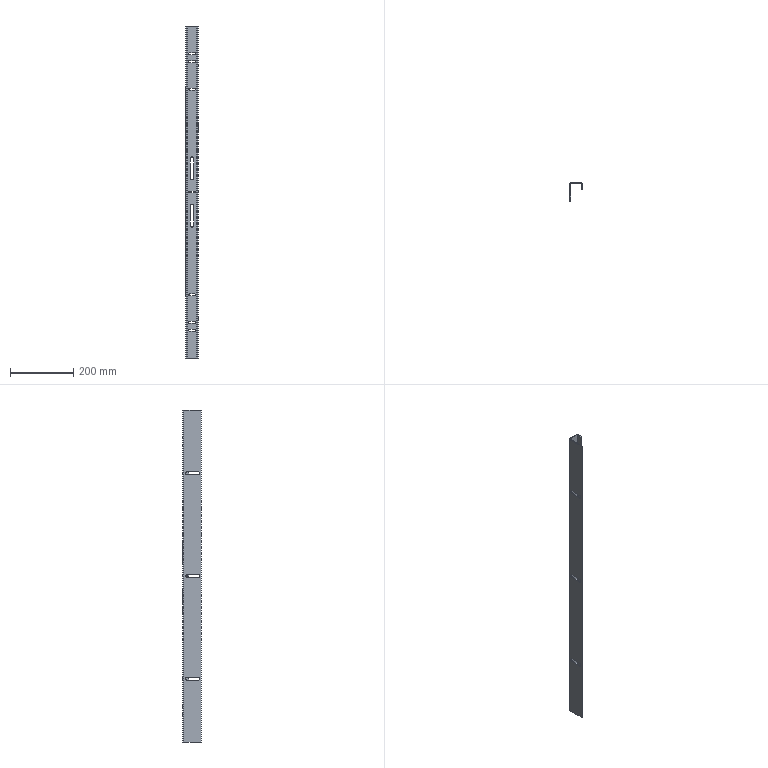Part | 1 solid | 87 faces | box 38.5 x 60 x 1050 mm | volume 335852 mm3 | cylinder 45 | plane 42 | commonest cylinder face diameters 6 x31 10 x6 12 x4 2 x2 8 x2